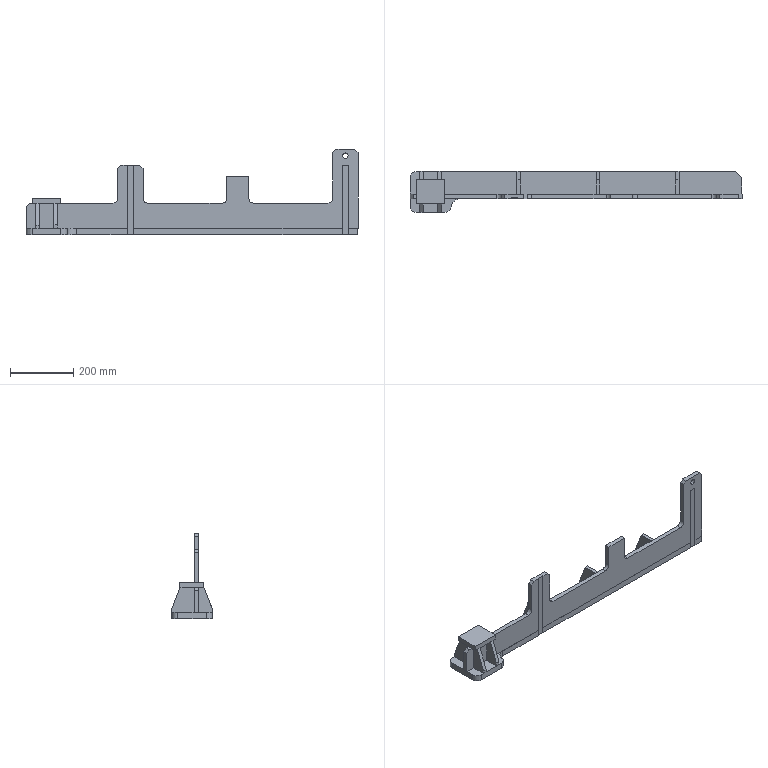Part | STEP file | Backup 2012-3-22-07 | 1 solid | 102 faces | box 1050 x 130.1 x 270 mm | volume 3935848 mm3 | plane 91 | cylinder 11 | commonest cylinder face diameters 30 x5 40 x3 17 x2 60 x1